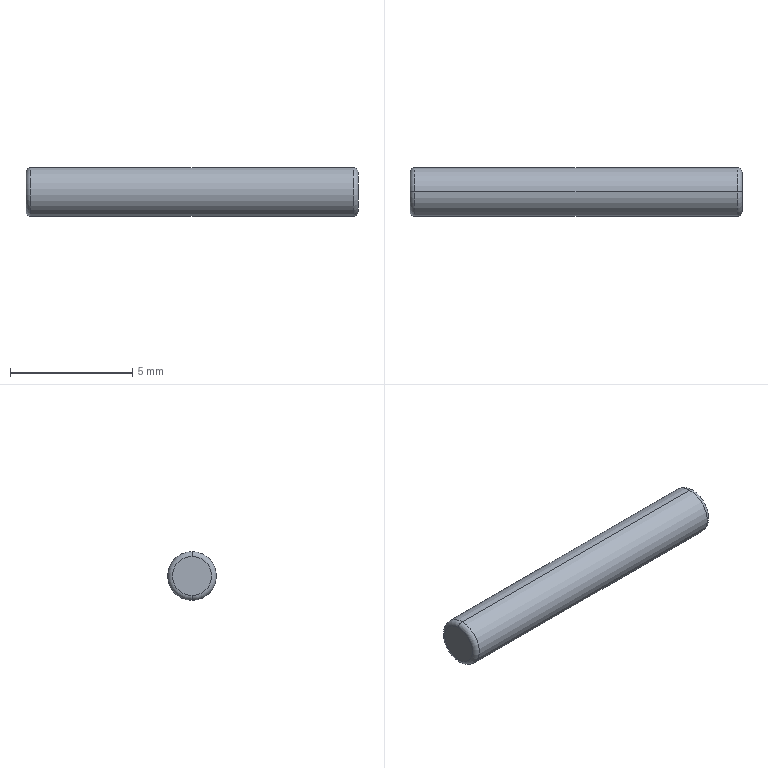Part | SolidWorks | features Extrusion 1, Fillet 1 | 1 solid | 8 faces | box 13.6 x 2 x 2 mm | volume 42.623 mm3 | torus 4 | cylinder 2 | plane 2 | commonest cylinder face diameters 2 x2
STEP:
#1=CARTESIAN_POINT('',(-6.8,0.,0.8));
#2=VERTEX_POINT('',#1);
#3=CARTESIAN_POINT('',(-6.8,0.,-0.8));
#4=VERTEX_POINT('',#3);
#5=CARTESIAN_POINT('',(-6.8,0.,0.));
#6=DIRECTION('',(-1.,0.,0.));
#7=DIRECTION('',(0.,0.,-1.));
#8=AXIS2_PLACEMENT_3D('',#5,#6,#7);
#9=CIRCLE('',#8,0.8);
#10=EDGE_CURVE('',#2,#4,#9,.T.);
#11=ORIENTED_EDGE('',*,*,#10,.F.);
#12=CARTESIAN_POINT('',(-6.6,0.,1.));
#13=VERTEX_POINT('',#12);
#14=CARTESIAN_POINT('',(-6.6,0.,0.8));
#15=DIRECTION('',(0.,1.,0.));
#16=DIRECTION('',(0.,0.,1.));
#17=AXIS2_PLACEMENT_3D('',#14,#15,#16);
#18=CIRCLE('',#17,0.2);
#19=EDGE_CURVE('',#2,#13,#18,.T.);
#20=ORIENTED_EDGE('',*,*,#19,.T.);
#21=CARTESIAN_POINT('',(-6.6,0.,-1.));
#22=VERTEX_POINT('',#21);
#23=CARTESIAN_POINT('',(-6.6,0.,0.));
#24=DIRECTION('',(1.,0.,0.));
#25=DIRECTION('',(0.,0.,-1.));
#26=AXIS2_PLACEMENT_3D('',#23,#24,#25);
#27=CIRCLE('',#26,1.);
#28=EDGE_CURVE('',#22,#13,#27,.T.);
#29=ORIENTED_EDGE('',*,*,#28,.F.);
#30=CARTESIAN_POINT('',(-6.6,0.,-0.8));
#31=DIRECTION('',(0.,-1.,0.));
#32=DIRECTION('',(0.,0.,-1.));
#33=AXIS2_PLACEMENT_3D('',#30,#31,#32);
#34=CIRCLE('',#33,0.2);
#35=EDGE_CURVE('',#4,#22,#34,.T.);
#36=ORIENTED_EDGE('',*,*,#35,.F.);
#37=EDGE_LOOP('',(#11,#20,#29,#36));
#38=FACE_OUTER_BOUND('',#37,.T.);
#39=CARTESIAN_POINT('',(-6.6,0.,0.));
#40=DIRECTION('',(1.,0.,0.));
#41=DIRECTION('',(0.,0.,-1.));
#42=AXIS2_PLACEMENT_3D('',#39,#40,#41);
#43=TOROIDAL_SURFACE('',#42,0.8,0.2);
#44=ADVANCED_FACE('',(#38),#43,.T.);
#45=CARTESIAN_POINT('',(6.6,0.,1.));
#46=VERTEX_POINT('',#45);
#47=CARTESIAN_POINT('',(6.6,0.,-1.));
#48=VERTEX_POINT('',#47);
#49=CARTESIAN_POINT('',(6.6,0.,0.));
#50=DIRECTION('',(-1.,0.,0.));
#51=DIRECTION('',(0.,0.,-1.));
#52=AXIS2_PLACEMENT_3D('',#49,#50,#51);
#53=CIRCLE('',#52,1.);
#54=EDGE_CURVE('',#46,#48,#53,.T.);
#55=ORIENTED_EDGE('',*,*,#54,.F.);
#56=CARTESIAN_POINT('',(6.8,0.,0.8));
#57=VERTEX_POINT('',#56);
#58=CARTESIAN_POINT('',(6.6,0.,0.8));
#59=DIRECTION('',(0.,1.,0.));
#60=DIRECTION('',(0.,0.,1.));
#61=AXIS2_PLACEMENT_3D('',#58,#59,#60);
#62=CIRCLE('',#61,0.2);
#63=EDGE_CURVE('',#46,#57,#62,.T.);
#64=ORIENTED_EDGE('',*,*,#63,.T.);
#65=CARTESIAN_POINT('',(6.8,0.,-0.8));
#66=VERTEX_POINT('',#65);
#67=CARTESIAN_POINT('',(6.8,0.,0.));
#68=DIRECTION('',(1.,0.,0.));
#69=DIRECTION('',(0.,0.,-1.));
#70=AXIS2_PLACEMENT_3D('',#67,#68,#69);
#71=CIRCLE('',#70,0.8);
#72=EDGE_CURVE('',#66,#57,#71,.T.);
#73=ORIENTED_EDGE('',*,*,#72,.F.);
#74=CARTESIAN_POINT('',(6.6,0.,-0.8));
#75=DIRECTION('',(0.,-1.,0.));
#76=DIRECTION('',(0.,0.,-1.));
#77=AXIS2_PLACEMENT_3D('',#74,#75,#76);
#78=CIRCLE('',#77,0.2);
#79=EDGE_CURVE('',#48,#66,#78,.T.);
#80=ORIENTED_EDGE('',*,*,#79,.F.);
#81=EDGE_LOOP('',(#55,#64,#73,#80));
#82=FACE_OUTER_BOUND('',#81,.T.);
#83=CARTESIAN_POINT('',(6.6,0.,0.));
#84=DIRECTION('',(1.,0.,0.));
#85=DIRECTION('',(0.,0.,-1.));
#86=AXIS2_PLACEMENT_3D('',#83,#84,#85);
#87=TOROIDAL_SURFACE('',#86,0.8,0.2);
#88=ADVANCED_FACE('',(#82),#87,.T.);
#89=ORIENTED_EDGE('',*,*,#54,.T.);
#90=CARTESIAN_POINT('',(6.8,0.,-1.));
#91=DIRECTION('',(-1.,0.,0.));
#92=VECTOR('',#91,1000.);
#93=LINE('',#90,#92);
#94=EDGE_CURVE('',#48,#22,#93,.T.);
#95=ORIENTED_EDGE('',*,*,#94,.T.);
#96=ORIENTED_EDGE('',*,*,#28,.T.);
#97=CARTESIAN_POINT('',(6.8,0.,1.));
#98=DIRECTION('',(-1.,0.,0.));
#99=VECTOR('',#98,1000.);
#100=LINE('',#97,#99);
#101=EDGE_CURVE('',#46,#13,#100,.T.);
#102=ORIENTED_EDGE('',*,*,#101,.F.);
#103=EDGE_LOOP('',(#89,#95,#96,#102));
#104=FACE_OUTER_BOUND('',#103,.T.);
#105=CARTESIAN_POINT('',(6.8,0.,0.));
#106=DIRECTION('',(-1.,0.,0.));
#107=DIRECTION('',(0.,0.,1.));
#108=AXIS2_PLACEMENT_3D('',#105,#106,#107);
#109=CYLINDRICAL_SURFACE('',#108,1.);
#110=ADVANCED_FACE('',(#104),#109,.T.);
#111=ORIENTED_EDGE('',*,*,#94,.F.);
#112=CARTESIAN_POINT('',(6.6,0.,0.));
#113=DIRECTION('',(-1.,0.,0.));
#114=DIRECTION('',(0.,0.,-1.));
#115=AXIS2_PLACEMENT_3D('',#112,#113,#114);
#116=CIRCLE('',#115,1.);
#117=EDGE_CURVE('',#48,#46,#116,.T.);
#118=ORIENTED_EDGE('',*,*,#117,.T.);
#119=ORIENTED_EDGE('',*,*,#101,.T.);
#120=CARTESIAN_POINT('',(-6.6,0.,0.));
#121=DIRECTION('',(1.,0.,0.));
#122=DIRECTION('',(0.,0.,-1.));
#123=AXIS2_PLACEMENT_3D('',#120,#121,#122);
#124=CIRCLE('',#123,1.);
#125=EDGE_CURVE('',#13,#22,#124,.T.);
#126=ORIENTED_EDGE('',*,*,#125,.T.);
#127=EDGE_LOOP('',(#111,#118,#119,#126));
#128=FACE_OUTER_BOUND('',#127,.T.);
#129=CARTESIAN_POINT('',(6.8,0.,0.));
#130=DIRECTION('',(-1.,0.,0.));
#131=DIRECTION('',(0.,0.,1.));
#132=AXIS2_PLACEMENT_3D('',#129,#130,#131);
#133=CYLINDRICAL_SURFACE('',#132,1.);
#134=ADVANCED_FACE('',(#128),#133,.T.);
#135=ORIENTED_EDGE('',*,*,#72,.T.);
#136=CARTESIAN_POINT('',(6.8,0.,0.));
#137=DIRECTION('',(1.,0.,0.));
#138=DIRECTION('',(0.,0.,-1.));
#139=AXIS2_PLACEMENT_3D('',#136,#137,#138);
#140=CIRCLE('',#139,0.8);
#141=EDGE_CURVE('',#57,#66,#140,.T.);
#142=ORIENTED_EDGE('',*,*,#141,.T.);
#143=EDGE_LOOP('',(#135,#142));
#144=FACE_OUTER_BOUND('',#143,.T.);
#145=CARTESIAN_POINT('',(6.8,0.,0.));
#146=DIRECTION('',(1.,0.,0.));
#147=DIRECTION('',(0.,0.,-1.));
#148=AXIS2_PLACEMENT_3D('',#145,#146,#147);
#149=PLANE('',#148);
#150=ADVANCED_FACE('',(#144),#149,.T.);
#151=CARTESIAN_POINT('',(-6.8,0.,0.));
#152=DIRECTION('',(-1.,0.,0.));
#153=DIRECTION('',(0.,0.,-1.));
#154=AXIS2_PLACEMENT_3D('',#151,#152,#153);
#155=CIRCLE('',#154,0.8);
#156=EDGE_CURVE('',#4,#2,#155,.T.);
#157=ORIENTED_EDGE('',*,*,#156,.T.);
#158=ORIENTED_EDGE('',*,*,#10,.T.);
#159=EDGE_LOOP('',(#157,#158));
#160=FACE_OUTER_BOUND('',#159,.T.);
#161=CARTESIAN_POINT('',(-6.8,0.,0.));
#162=DIRECTION('',(1.,0.,0.));
#163=DIRECTION('',(0.,0.,-1.));
#164=AXIS2_PLACEMENT_3D('',#161,#162,#163);
#165=PLANE('',#164);
#166=ADVANCED_FACE('',(#160),#165,.F.);
#167=ORIENTED_EDGE('',*,*,#63,.F.);
#168=ORIENTED_EDGE('',*,*,#117,.F.);
#169=ORIENTED_EDGE('',*,*,#79,.T.);
#170=ORIENTED_EDGE('',*,*,#141,.F.);
#171=EDGE_LOOP('',(#167,#168,#169,#170));
#172=FACE_OUTER_BOUND('',#171,.T.);
#173=CARTESIAN_POINT('',(6.6,0.,0.));
#174=DIRECTION('',(1.,0.,0.));
#175=DIRECTION('',(0.,0.,-1.));
#176=AXIS2_PLACEMENT_3D('',#173,#174,#175);
#177=TOROIDAL_SURFACE('',#176,0.8,0.2);
#178=ADVANCED_FACE('',(#172),#177,.T.);
#179=ORIENTED_EDGE('',*,*,#19,.F.);
#180=ORIENTED_EDGE('',*,*,#156,.F.);
#181=ORIENTED_EDGE('',*,*,#35,.T.);
#182=ORIENTED_EDGE('',*,*,#125,.F.);
#183=EDGE_LOOP('',(#179,#180,#181,#182));
#184=FACE_OUTER_BOUND('',#183,.T.);
#185=CARTESIAN_POINT('',(-6.6,0.,0.));
#186=DIRECTION('',(1.,0.,0.));
#187=DIRECTION('',(0.,0.,-1.));
#188=AXIS2_PLACEMENT_3D('',#185,#186,#187);
#189=TOROIDAL_SURFACE('',#188,0.8,0.2);
#190=ADVANCED_FACE('',(#184),#189,.T.);
#191=CLOSED_SHELL('',(#44,#88,#110,#134,#150,#166,#178,#190));
#192=MANIFOLD_SOLID_BREP('',#191);
#193=CARTESIAN_POINT('',(0.,0.,0.));
#194=DIRECTION('',(0.,0.,1.));
#195=DIRECTION('',(1.,0.,0.));
#196=AXIS2_PLACEMENT_3D('',#193,#194,#195);
#197=(LENGTH_UNIT()NAMED_UNIT(*)SI_UNIT(.MILLI.,.METRE.));
#198=UNCERTAINTY_MEASURE_WITH_UNIT(LENGTH_MEASURE(0.00001),#197,'','');
#199=(NAMED_UNIT(*)PLANE_ANGLE_UNIT()SI_UNIT($,.RADIAN.));
#200=(NAMED_UNIT(*)SI_UNIT($,.STERADIAN.)SOLID_ANGLE_UNIT());
#201=(GEOMETRIC_REPRESENTATION_CONTEXT(3)GLOBAL_UNCERTAINTY_ASSIGNED_CONTEXT((#198))GLOBAL_UNIT_ASSIGNED_CONTEXT((#197,#199,#200))REPRESENTATION_CONTEXT('',''));
#202=ADVANCED_BREP_SHAPE_REPRESENTATION('',(#192,#196),#201);